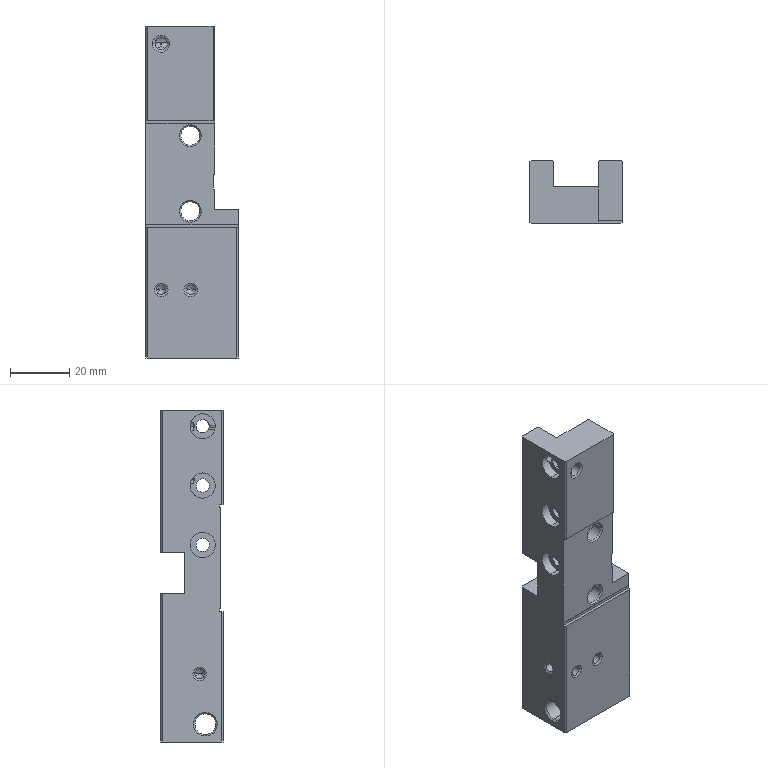Part | NX | 1 solid | 148 faces | box 31.2 x 21.2 x 112 mm | volume 41242 mm3 | cone 57 | cylinder 48 | plane 43 | commonest cylinder face diameters 3.3 x16 2.5 x8 4.5 x6 8.5 x6 6.4 x4 11 x4